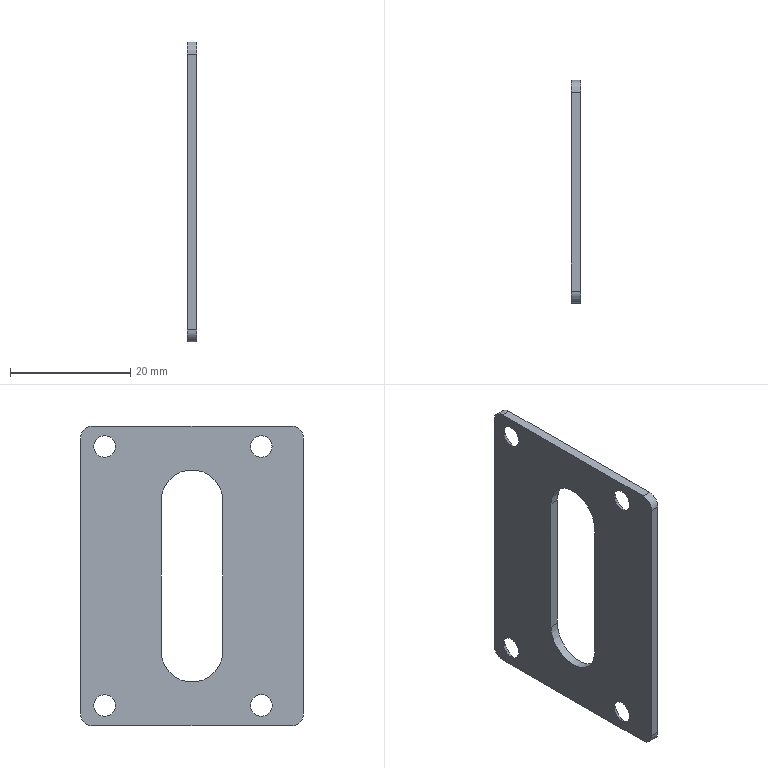Part | SolidWorks | features BaseBody 1, ICE 1 | 1 solid | 22 faces | box 1.5 x 37 x 49.8 mm | volume 2125 mm3 | cone 8 | plane 8 | cylinder 6 | commonest cylinder face diameters 4 x4 10.246 x2
STEP:
#1=CARTESIAN_POINT('',(0.,-2.2,3.4));
#2=VERTEX_POINT('',#1);
#3=CARTESIAN_POINT('',(0.,-5.8,3.4));
#4=VERTEX_POINT('',#3);
#5=CARTESIAN_POINT('',(0.,-4.,3.4));
#6=DIRECTION('',(-1.,0.,0.));
#7=DIRECTION('',(0.,1.,0.));
#8=AXIS2_PLACEMENT_3D('',#5,#6,#7);
#9=CIRCLE('',#8,1.8);
#10=EDGE_CURVE('',#2,#4,#9,.T.);
#11=ORIENTED_EDGE('',*,*,#10,.T.);
#12=CARTESIAN_POINT('',(1.5,-7.3,3.4));
#13=VERTEX_POINT('',#12);
#14=CARTESIAN_POINT('',(1.5,-7.3,3.4));
#15=DIRECTION('',(0.7071,-0.7071,0.));
#16=VECTOR('',#15,1000.);
#17=LINE('',#14,#16);
#18=EDGE_CURVE('',#4,#13,#17,.T.);
#19=ORIENTED_EDGE('',*,*,#18,.T.);
#20=CARTESIAN_POINT('',(1.5,-0.7,3.4));
#21=VERTEX_POINT('',#20);
#22=CARTESIAN_POINT('',(1.5,-4.,3.4));
#23=DIRECTION('',(-1.,0.,0.));
#24=DIRECTION('',(0.,1.,0.));
#25=AXIS2_PLACEMENT_3D('',#22,#23,#24);
#26=CIRCLE('',#25,3.3);
#27=EDGE_CURVE('',#21,#13,#26,.T.);
#28=ORIENTED_EDGE('',*,*,#27,.F.);
#29=CARTESIAN_POINT('',(1.5,-0.7,3.4));
#30=DIRECTION('',(0.7071,0.7071,0.));
#31=VECTOR('',#30,1000.);
#32=LINE('',#29,#31);
#33=EDGE_CURVE('',#2,#21,#32,.T.);
#34=ORIENTED_EDGE('',*,*,#33,.F.);
#35=EDGE_LOOP('',(#11,#19,#28,#34));
#36=FACE_OUTER_BOUND('',#35,.T.);
#37=CARTESIAN_POINT('',(1.5,-4.,3.4));
#38=DIRECTION('',(1.,0.,0.));
#39=DIRECTION('',(0.,1.,0.));
#40=AXIS2_PLACEMENT_3D('',#37,#38,#39);
#41=CONICAL_SURFACE('',#40,3.3,0.7854);
#42=ADVANCED_FACE('',(#36),#41,.F.);
#43=CARTESIAN_POINT('',(0.,-2.2,46.4));
#44=VERTEX_POINT('',#43);
#45=CARTESIAN_POINT('',(0.,-5.8,46.4));
#46=VERTEX_POINT('',#45);
#47=CARTESIAN_POINT('',(0.,-4.,46.4));
#48=DIRECTION('',(-1.,0.,0.));
#49=DIRECTION('',(0.,1.,0.));
#50=AXIS2_PLACEMENT_3D('',#47,#48,#49);
#51=CIRCLE('',#50,1.8);
#52=EDGE_CURVE('',#44,#46,#51,.T.);
#53=ORIENTED_EDGE('',*,*,#52,.T.);
#54=CARTESIAN_POINT('',(1.5,-7.3,46.4));
#55=VERTEX_POINT('',#54);
#56=CARTESIAN_POINT('',(1.5,-7.3,46.4));
#57=DIRECTION('',(0.7071,-0.7071,0.));
#58=VECTOR('',#57,1000.);
#59=LINE('',#56,#58);
#60=EDGE_CURVE('',#46,#55,#59,.T.);
#61=ORIENTED_EDGE('',*,*,#60,.T.);
#62=CARTESIAN_POINT('',(1.5,-0.7,46.4));
#63=VERTEX_POINT('',#62);
#64=CARTESIAN_POINT('',(1.5,-4.,46.4));
#65=DIRECTION('',(-1.,0.,0.));
#66=DIRECTION('',(0.,1.,0.));
#67=AXIS2_PLACEMENT_3D('',#64,#65,#66);
#68=CIRCLE('',#67,3.3);
#69=EDGE_CURVE('',#63,#55,#68,.T.);
#70=ORIENTED_EDGE('',*,*,#69,.F.);
#71=CARTESIAN_POINT('',(1.5,-0.7,46.4));
#72=DIRECTION('',(0.7071,0.7071,0.));
#73=VECTOR('',#72,1000.);
#74=LINE('',#71,#73);
#75=EDGE_CURVE('',#44,#63,#74,.T.);
#76=ORIENTED_EDGE('',*,*,#75,.F.);
#77=EDGE_LOOP('',(#53,#61,#70,#76));
#78=FACE_OUTER_BOUND('',#77,.T.);
#79=CARTESIAN_POINT('',(1.5,-4.,46.4));
#80=DIRECTION('',(1.,0.,0.));
#81=DIRECTION('',(0.,1.,0.));
#82=AXIS2_PLACEMENT_3D('',#79,#80,#81);
#83=CONICAL_SURFACE('',#82,3.3,0.7854);
#84=ADVANCED_FACE('',(#78),#83,.F.);
#85=CARTESIAN_POINT('',(0.,-28.2,46.4));
#86=VERTEX_POINT('',#85);
#87=CARTESIAN_POINT('',(0.,-31.8,46.4));
#88=VERTEX_POINT('',#87);
#89=CARTESIAN_POINT('',(0.,-30.,46.4));
#90=DIRECTION('',(-1.,0.,0.));
#91=DIRECTION('',(0.,1.,0.));
#92=AXIS2_PLACEMENT_3D('',#89,#90,#91);
#93=CIRCLE('',#92,1.8);
#94=EDGE_CURVE('',#86,#88,#93,.T.);
#95=ORIENTED_EDGE('',*,*,#94,.T.);
#96=CARTESIAN_POINT('',(1.5,-33.3,46.4));
#97=VERTEX_POINT('',#96);
#98=CARTESIAN_POINT('',(1.5,-33.3,46.4));
#99=DIRECTION('',(0.7071,-0.7071,0.));
#100=VECTOR('',#99,1000.);
#101=LINE('',#98,#100);
#102=EDGE_CURVE('',#88,#97,#101,.T.);
#103=ORIENTED_EDGE('',*,*,#102,.T.);
#104=CARTESIAN_POINT('',(1.5,-26.7,46.4));
#105=VERTEX_POINT('',#104);
#106=CARTESIAN_POINT('',(1.5,-30.,46.4));
#107=DIRECTION('',(-1.,0.,0.));
#108=DIRECTION('',(0.,1.,0.));
#109=AXIS2_PLACEMENT_3D('',#106,#107,#108);
#110=CIRCLE('',#109,3.3);
#111=EDGE_CURVE('',#105,#97,#110,.T.);
#112=ORIENTED_EDGE('',*,*,#111,.F.);
#113=CARTESIAN_POINT('',(1.5,-26.7,46.4));
#114=DIRECTION('',(0.7071,0.7071,0.));
#115=VECTOR('',#114,1000.);
#116=LINE('',#113,#115);
#117=EDGE_CURVE('',#86,#105,#116,.T.);
#118=ORIENTED_EDGE('',*,*,#117,.F.);
#119=EDGE_LOOP('',(#95,#103,#112,#118));
#120=FACE_OUTER_BOUND('',#119,.T.);
#121=CARTESIAN_POINT('',(1.5,-30.,46.4));
#122=DIRECTION('',(1.,0.,0.));
#123=DIRECTION('',(0.,1.,0.));
#124=AXIS2_PLACEMENT_3D('',#121,#122,#123);
#125=CONICAL_SURFACE('',#124,3.3,0.7854);
#126=ADVANCED_FACE('',(#120),#125,.F.);
#127=CARTESIAN_POINT('',(0.,-30.,1.6));
#128=VERTEX_POINT('',#127);
#129=CARTESIAN_POINT('',(0.,-30.,5.2));
#130=VERTEX_POINT('',#129);
#131=CARTESIAN_POINT('',(0.,-30.,3.4));
#132=DIRECTION('',(-1.,0.,0.));
#133=DIRECTION('',(0.,0.,-1.));
#134=AXIS2_PLACEMENT_3D('',#131,#132,#133);
#135=CIRCLE('',#134,1.8);
#136=EDGE_CURVE('',#128,#130,#135,.T.);
#137=ORIENTED_EDGE('',*,*,#136,.T.);
#138=CARTESIAN_POINT('',(1.5,-30.,6.7));
#139=VERTEX_POINT('',#138);
#140=CARTESIAN_POINT('',(1.5,-30.,6.7));
#141=DIRECTION('',(0.7071,0.,0.7071));
#142=VECTOR('',#141,1000.);
#143=LINE('',#140,#142);
#144=EDGE_CURVE('',#130,#139,#143,.T.);
#145=ORIENTED_EDGE('',*,*,#144,.T.);
#146=CARTESIAN_POINT('',(1.5,-30.,0.1));
#147=VERTEX_POINT('',#146);
#148=CARTESIAN_POINT('',(1.5,-30.,3.4));
#149=DIRECTION('',(-1.,0.,0.));
#150=DIRECTION('',(0.,0.,-1.));
#151=AXIS2_PLACEMENT_3D('',#148,#149,#150);
#152=CIRCLE('',#151,3.3);
#153=EDGE_CURVE('',#147,#139,#152,.T.);
#154=ORIENTED_EDGE('',*,*,#153,.F.);
#155=CARTESIAN_POINT('',(1.5,-30.,0.1));
#156=DIRECTION('',(0.7071,0.,-0.7071));
#157=VECTOR('',#156,1000.);
#158=LINE('',#155,#157);
#159=EDGE_CURVE('',#128,#147,#158,.T.);
#160=ORIENTED_EDGE('',*,*,#159,.F.);
#161=EDGE_LOOP('',(#137,#145,#154,#160));
#162=FACE_OUTER_BOUND('',#161,.T.);
#163=CARTESIAN_POINT('',(1.5,-30.,3.4));
#164=DIRECTION('',(1.,0.,0.));
#165=DIRECTION('',(0.,0.,-1.));
#166=AXIS2_PLACEMENT_3D('',#163,#164,#165);
#167=CONICAL_SURFACE('',#166,3.3,0.7854);
#168=ADVANCED_FACE('',(#162),#167,.F.);
#169=CARTESIAN_POINT('',(0.,-13.377,12.4));
#170=VERTEX_POINT('',#169);
#171=CARTESIAN_POINT('',(0.,-13.377,37.4));
#172=VERTEX_POINT('',#171);
#173=CARTESIAN_POINT('',(0.,-13.377,37.4));
#174=DIRECTION('',(0.,0.,1.));
#175=VECTOR('',#174,1000.);
#176=LINE('',#173,#175);
#177=EDGE_CURVE('',#170,#172,#176,.T.);
#178=ORIENTED_EDGE('',*,*,#177,.T.);
#179=CARTESIAN_POINT('',(0.,-23.623,37.4));
#180=VERTEX_POINT('',#179);
#181=CARTESIAN_POINT('',(0.,-18.5,37.4));
#182=DIRECTION('',(1.,0.,0.));
#183=DIRECTION('',(0.,1.,0.));
#184=AXIS2_PLACEMENT_3D('',#181,#182,#183);
#185=CIRCLE('',#184,5.123);
#186=EDGE_CURVE('',#172,#180,#185,.T.);
#187=ORIENTED_EDGE('',*,*,#186,.T.);
#188=CARTESIAN_POINT('',(0.,-23.623,12.4));
#189=VERTEX_POINT('',#188);
#190=CARTESIAN_POINT('',(0.,-23.623,37.4));
#191=DIRECTION('',(0.,0.,-1.));
#192=VECTOR('',#191,1000.);
#193=LINE('',#190,#192);
#194=EDGE_CURVE('',#180,#189,#193,.T.);
#195=ORIENTED_EDGE('',*,*,#194,.T.);
#196=CARTESIAN_POINT('',(0.,-18.5,12.4));
#197=DIRECTION('',(1.,0.,0.));
#198=DIRECTION('',(0.,1.,0.));
#199=AXIS2_PLACEMENT_3D('',#196,#197,#198);
#200=CIRCLE('',#199,5.123);
#201=EDGE_CURVE('',#189,#170,#200,.T.);
#202=ORIENTED_EDGE('',*,*,#201,.T.);
#203=EDGE_LOOP('',(#178,#187,#195,#202));
#204=FACE_BOUND('',#203,.T.);
#205=CARTESIAN_POINT('',(0.,-37.,2.));
#206=VERTEX_POINT('',#205);
#207=CARTESIAN_POINT('',(0.,-35.,0.));
#208=VERTEX_POINT('',#207);
#209=CARTESIAN_POINT('',(0.,-35.,2.));
#210=DIRECTION('',(1.,0.,0.));
#211=DIRECTION('',(0.,0.,1.));
#212=AXIS2_PLACEMENT_3D('',#209,#210,#211);
#213=CIRCLE('',#212,2.);
#214=EDGE_CURVE('',#206,#208,#213,.T.);
#215=ORIENTED_EDGE('',*,*,#214,.F.);
#216=CARTESIAN_POINT('',(0.,-37.,47.8));
#217=VERTEX_POINT('',#216);
#218=CARTESIAN_POINT('',(0.,-37.,49.8));
#219=DIRECTION('',(0.,0.,-1.));
#220=VECTOR('',#219,1000.);
#221=LINE('',#218,#220);
#222=EDGE_CURVE('',#217,#206,#221,.T.);
#223=ORIENTED_EDGE('',*,*,#222,.F.);
#224=CARTESIAN_POINT('',(0.,-35.,49.8));
#225=VERTEX_POINT('',#224);
#226=CARTESIAN_POINT('',(0.,-35.,47.8));
#227=DIRECTION('',(1.,0.,0.));
#228=DIRECTION('',(0.,0.,-1.));
#229=AXIS2_PLACEMENT_3D('',#226,#227,#228);
#230=CIRCLE('',#229,2.);
#231=EDGE_CURVE('',#225,#217,#230,.T.);
#232=ORIENTED_EDGE('',*,*,#231,.F.);
#233=CARTESIAN_POINT('',(0.,-2.,49.8));
#234=VERTEX_POINT('',#233);
#235=CARTESIAN_POINT('',(0.,-37.,49.8));
#236=DIRECTION('',(0.,-1.,0.));
#237=VECTOR('',#236,1000.);
#238=LINE('',#235,#237);
#239=EDGE_CURVE('',#234,#225,#238,.T.);
#240=ORIENTED_EDGE('',*,*,#239,.F.);
#241=CARTESIAN_POINT('',(0.,0.,47.8));
#242=VERTEX_POINT('',#241);
#243=CARTESIAN_POINT('',(0.,-2.,47.8));
#244=DIRECTION('',(1.,0.,0.));
#245=DIRECTION('',(0.,-1.,0.));
#246=AXIS2_PLACEMENT_3D('',#243,#244,#245);
#247=CIRCLE('',#246,2.);
#248=EDGE_CURVE('',#242,#234,#247,.T.);
#249=ORIENTED_EDGE('',*,*,#248,.F.);
#250=CARTESIAN_POINT('',(0.,0.,2.));
#251=VERTEX_POINT('',#250);
#252=CARTESIAN_POINT('',(0.,0.,49.8));
#253=DIRECTION('',(0.,0.,1.));
#254=VECTOR('',#253,1000.);
#255=LINE('',#252,#254);
#256=EDGE_CURVE('',#251,#242,#255,.T.);
#257=ORIENTED_EDGE('',*,*,#256,.F.);
#258=CARTESIAN_POINT('',(0.,-2.,0.));
#259=VERTEX_POINT('',#258);
#260=CARTESIAN_POINT('',(0.,-2.,2.));
#261=DIRECTION('',(1.,0.,0.));
#262=DIRECTION('',(0.,1.,0.));
#263=AXIS2_PLACEMENT_3D('',#260,#261,#262);
#264=CIRCLE('',#263,2.);
#265=EDGE_CURVE('',#259,#251,#264,.T.);
#266=ORIENTED_EDGE('',*,*,#265,.F.);
#267=CARTESIAN_POINT('',(0.,-37.,0.));
#268=DIRECTION('',(0.,1.,0.));
#269=VECTOR('',#268,1000.);
#270=LINE('',#267,#269);
#271=EDGE_CURVE('',#208,#259,#270,.T.);
#272=ORIENTED_EDGE('',*,*,#271,.F.);
#273=EDGE_LOOP('',(#215,#223,#232,#240,#249,#257,#266,#272));
#274=FACE_OUTER_BOUND('',#273,.T.);
#275=ORIENTED_EDGE('',*,*,#10,.F.);
#276=CARTESIAN_POINT('',(0.,-4.,3.4));
#277=DIRECTION('',(-1.,0.,0.));
#278=DIRECTION('',(0.,1.,0.));
#279=AXIS2_PLACEMENT_3D('',#276,#277,#278);
#280=CIRCLE('',#279,1.8);
#281=EDGE_CURVE('',#4,#2,#280,.T.);
#282=ORIENTED_EDGE('',*,*,#281,.F.);
#283=EDGE_LOOP('',(#275,#282));
#284=FACE_BOUND('',#283,.T.);
#285=ORIENTED_EDGE('',*,*,#52,.F.);
#286=CARTESIAN_POINT('',(0.,-4.,46.4));
#287=DIRECTION('',(-1.,0.,0.));
#288=DIRECTION('',(0.,1.,0.));
#289=AXIS2_PLACEMENT_3D('',#286,#287,#288);
#290=CIRCLE('',#289,1.8);
#291=EDGE_CURVE('',#46,#44,#290,.T.);
#292=ORIENTED_EDGE('',*,*,#291,.F.);
#293=EDGE_LOOP('',(#285,#292));
#294=FACE_BOUND('',#293,.T.);
#295=ORIENTED_EDGE('',*,*,#94,.F.);
#296=CARTESIAN_POINT('',(0.,-30.,46.4));
#297=DIRECTION('',(-1.,0.,0.));
#298=DIRECTION('',(0.,1.,0.));
#299=AXIS2_PLACEMENT_3D('',#296,#297,#298);
#300=CIRCLE('',#299,1.8);
#301=EDGE_CURVE('',#88,#86,#300,.T.);
#302=ORIENTED_EDGE('',*,*,#301,.F.);
#303=EDGE_LOOP('',(#295,#302));
#304=FACE_BOUND('',#303,.T.);
#305=ORIENTED_EDGE('',*,*,#136,.F.);
#306=CARTESIAN_POINT('',(0.,-30.,3.4));
#307=DIRECTION('',(-1.,0.,0.));
#308=DIRECTION('',(0.,0.,-1.));
#309=AXIS2_PLACEMENT_3D('',#306,#307,#308);
#310=CIRCLE('',#309,1.8);
#311=EDGE_CURVE('',#130,#128,#310,.T.);
#312=ORIENTED_EDGE('',*,*,#311,.F.);
#313=EDGE_LOOP('',(#305,#312));
#314=FACE_BOUND('',#313,.T.);
#315=CARTESIAN_POINT('',(0.,-37.,49.8));
#316=DIRECTION('',(1.,0.,0.));
#317=DIRECTION('',(0.,1.,0.));
#318=AXIS2_PLACEMENT_3D('',#315,#316,#317);
#319=PLANE('',#318);
#320=ADVANCED_FACE('',(#204,#274,#284,#294,#304,#314),#319,.F.);
#321=ORIENTED_EDGE('',*,*,#271,.T.);
#322=CARTESIAN_POINT('',(1.5,-2.,0.));
#323=VERTEX_POINT('',#322);
#324=CARTESIAN_POINT('',(0.,-2.,0.));
#325=DIRECTION('',(1.,0.,0.));
#326=VECTOR('',#325,1000.);
#327=LINE('',#324,#326);
#328=EDGE_CURVE('',#259,#323,#327,.T.);
#329=ORIENTED_EDGE('',*,*,#328,.T.);
#330=CARTESIAN_POINT('',(1.5,-35.,0.));
#331=VERTEX_POINT('',#330);
#332=CARTESIAN_POINT('',(1.5,0.,0.));
#333=DIRECTION('',(0.,-1.,0.));
#334=VECTOR('',#333,1000.);
#335=LINE('',#332,#334);
#336=EDGE_CURVE('',#323,#331,#335,.T.);
#337=ORIENTED_EDGE('',*,*,#336,.T.);
#338=CARTESIAN_POINT('',(0.,-35.,0.));
#339=DIRECTION('',(-1.,0.,0.));
#340=VECTOR('',#339,1000.);
#341=LINE('',#338,#340);
#342=EDGE_CURVE('',#331,#208,#341,.T.);
#343=ORIENTED_EDGE('',*,*,#342,.T.);
#344=EDGE_LOOP('',(#321,#329,#337,#343));
#345=FACE_OUTER_BOUND('',#344,.T.);
#346=CARTESIAN_POINT('',(0.,0.,0.));
#347=DIRECTION('',(0.,0.,-1.));
#348=DIRECTION('',(-1.,0.,0.));
#349=AXIS2_PLACEMENT_3D('',#346,#347,#348);
#350=PLANE('',#349);
#351=ADVANCED_FACE('',(#345),#350,.T.);
#352=CARTESIAN_POINT('',(1.5,-37.,2.));
#353=VERTEX_POINT('',#352);
#354=CARTESIAN_POINT('',(1.5,-35.,2.));
#355=DIRECTION('',(-1.,0.,0.));
#356=DIRECTION('',(0.,0.,1.));
#357=AXIS2_PLACEMENT_3D('',#354,#355,#356);
#358=CIRCLE('',#357,2.);
#359=EDGE_CURVE('',#331,#353,#358,.T.);
#360=ORIENTED_EDGE('',*,*,#359,.T.);
#361=CARTESIAN_POINT('',(1.5,-37.,2.));
#362=DIRECTION('',(-1.,0.,0.));
#363=VECTOR('',#362,1000.);
#364=LINE('',#361,#363);
#365=EDGE_CURVE('',#353,#206,#364,.T.);
#366=ORIENTED_EDGE('',*,*,#365,.T.);
#367=ORIENTED_EDGE('',*,*,#214,.T.);
#368=ORIENTED_EDGE('',*,*,#342,.F.);
#369=EDGE_LOOP('',(#360,#366,#367,#368));
#370=FACE_OUTER_BOUND('',#369,.T.);
#371=CARTESIAN_POINT('',(1.5,-35.,2.));
#372=DIRECTION('',(-1.,0.,0.));
#373=DIRECTION('',(0.,0.,1.));
#374=AXIS2_PLACEMENT_3D('',#371,#372,#373);
#375=CYLINDRICAL_SURFACE('',#374,2.);
#376=ADVANCED_FACE('',(#370),#375,.T.);
#377=ORIENTED_EDGE('',*,*,#365,.F.);
#378=CARTESIAN_POINT('',(1.5,-37.,47.8));
#379=VERTEX_POINT('',#378);
#380=CARTESIAN_POINT('',(1.5,-37.,49.8));
#381=DIRECTION('',(0.,0.,-1.));
#382=VECTOR('',#381,1000.);
#383=LINE('',#380,#382);
#384=EDGE_CURVE('',#379,#353,#383,.T.);
#385=ORIENTED_EDGE('',*,*,#384,.F.);
#386=CARTESIAN_POINT('',(1.5,-37.,47.8));
#387=DIRECTION('',(1.,0.,0.));
#388=VECTOR('',#387,1000.);
#389=LINE('',#386,#388);
#390=EDGE_CURVE('',#217,#379,#389,.T.);
#391=ORIENTED_EDGE('',*,*,#390,.F.);
#392=ORIENTED_EDGE('',*,*,#222,.T.);
#393=EDGE_LOOP('',(#377,#385,#391,#392));
#394=FACE_OUTER_BOUND('',#393,.T.);
#395=CARTESIAN_POINT('',(1.5,-37.,49.8));
#396=DIRECTION('',(0.,1.,0.));
#397=DIRECTION('',(0.,0.,1.));
#398=AXIS2_PLACEMENT_3D('',#395,#396,#397);
#399=PLANE('',#398);
#400=ADVANCED_FACE('',(#394),#399,.F.);
#401=CARTESIAN_POINT('',(1.5,-35.,49.8));
#402=VERTEX_POINT('',#401);
#403=CARTESIAN_POINT('',(1.5,-35.,47.8));
#404=DIRECTION('',(-1.,0.,0.));
#405=DIRECTION('',(0.,0.,-1.));
#406=AXIS2_PLACEMENT_3D('',#403,#404,#405);
#407=CIRCLE('',#406,2.);
#408=EDGE_CURVE('',#379,#402,#407,.T.);
#409=ORIENTED_EDGE('',*,*,#408,.T.);
#410=CARTESIAN_POINT('',(0.,-35.,49.8));
#411=DIRECTION('',(-1.,0.,0.));
#412=VECTOR('',#411,1000.);
#413=LINE('',#410,#412);
#414=EDGE_CURVE('',#402,#225,#413,.T.);
#415=ORIENTED_EDGE('',*,*,#414,.T.);
#416=ORIENTED_EDGE('',*,*,#231,.T.);
#417=ORIENTED_EDGE('',*,*,#390,.T.);
#418=EDGE_LOOP('',(#409,#415,#416,#417));
#419=FACE_OUTER_BOUND('',#418,.T.);
#420=CARTESIAN_POINT('',(0.,-35.,47.8));
#421=DIRECTION('',(1.,0.,0.));
#422=DIRECTION('',(0.,0.,-1.));
#423=AXIS2_PLACEMENT_3D('',#420,#421,#422);
#424=CYLINDRICAL_SURFACE('',#423,2.);
#425=ADVANCED_FACE('',(#419),#424,.T.);
#426=ORIENTED_EDGE('',*,*,#414,.F.);
#427=CARTESIAN_POINT('',(1.5,-2.,49.8));
#428=VERTEX_POINT('',#427);
#429=CARTESIAN_POINT('',(1.5,0.,49.8));
#430=DIRECTION('',(0.,-1.,0.));
#431=VECTOR('',#430,1000.);
#432=LINE('',#429,#431);
#433=EDGE_CURVE('',#428,#402,#432,.T.);
#434=ORIENTED_EDGE('',*,*,#433,.F.);
#435=CARTESIAN_POINT('',(0.,-2.,49.8));
#436=DIRECTION('',(1.,0.,0.));
#437=VECTOR('',#436,1000.);
#438=LINE('',#435,#437);
#439=EDGE_CURVE('',#234,#428,#438,.T.);
#440=ORIENTED_EDGE('',*,*,#439,.F.);
#441=ORIENTED_EDGE('',*,*,#239,.T.);
#442=EDGE_LOOP('',(#426,#434,#440,#441));
#443=FACE_OUTER_BOUND('',#442,.T.);
#444=CARTESIAN_POINT('',(0.,0.,49.8));
#445=DIRECTION('',(0.,0.,-1.));
#446=DIRECTION('',(-1.,0.,0.));
#447=AXIS2_PLACEMENT_3D('',#444,#445,#446);
#448=PLANE('',#447);
#449=ADVANCED_FACE('',(#443),#448,.F.);
#450=ORIENTED_EDGE('',*,*,#248,.T.);
#451=ORIENTED_EDGE('',*,*,#439,.T.);
#452=CARTESIAN_POINT('',(1.5,0.,47.8));
#453=VERTEX_POINT('',#452);
#454=CARTESIAN_POINT('',(1.5,-2.,47.8));
#455=DIRECTION('',(-1.,0.,0.));
#456=DIRECTION('',(0.,-1.,0.));
#457=AXIS2_PLACEMENT_3D('',#454,#455,#456);
#458=CIRCLE('',#457,2.);
#459=EDGE_CURVE('',#428,#453,#458,.T.);
#460=ORIENTED_EDGE('',*,*,#459,.T.);
#461=CARTESIAN_POINT('',(0.,0.,47.8));
#462=DIRECTION('',(-1.,0.,0.));
#463=VECTOR('',#462,1000.);
#464=LINE('',#461,#463);
#465=EDGE_CURVE('',#453,#242,#464,.T.);
#466=ORIENTED_EDGE('',*,*,#465,.T.);
#467=EDGE_LOOP('',(#450,#451,#460,#466));
#468=FACE_OUTER_BOUND('',#467,.T.);
#469=CARTESIAN_POINT('',(0.,-2.,47.8));
#470=DIRECTION('',(-1.,0.,0.));
#471=DIRECTION('',(0.,-1.,0.));
#472=AXIS2_PLACEMENT_3D('',#469,#470,#471);
#473=CYLINDRICAL_SURFACE('',#472,2.);
#474=ADVANCED_FACE('',(#468),#473,.T.);
#475=ORIENTED_EDGE('',*,*,#465,.F.);
#476=CARTESIAN_POINT('',(1.5,0.,2.));
#477=VERTEX_POINT('',#476);
#478=CARTESIAN_POINT('',(1.5,0.,49.8));
#479=DIRECTION('',(0.,0.,1.));
#480=VECTOR('',#479,1000.);
#481=LINE('',#478,#480);
#482=EDGE_CURVE('',#477,#453,#481,.T.);
#483=ORIENTED_EDGE('',*,*,#482,.F.);
#484=CARTESIAN_POINT('',(0.,0.,2.));
#485=DIRECTION('',(1.,0.,0.));
#486=VECTOR('',#485,1000.);
#487=LINE('',#484,#486);
#488=EDGE_CURVE('',#251,#477,#487,.T.);
#489=ORIENTED_EDGE('',*,*,#488,.F.);
#490=ORIENTED_EDGE('',*,*,#256,.T.);
#491=EDGE_LOOP('',(#475,#483,#489,#490));
#492=FACE_OUTER_BOUND('',#491,.T.);
#493=CARTESIAN_POINT('',(0.,0.,49.8));
#494=DIRECTION('',(0.,-1.,0.));
#495=DIRECTION('',(1.,0.,0.));
#496=AXIS2_PLACEMENT_3D('',#493,#494,#495);
#497=PLANE('',#496);
#498=ADVANCED_FACE('',(#492),#497,.F.);
#499=ORIENTED_EDGE('',*,*,#265,.T.);
#500=ORIENTED_EDGE('',*,*,#488,.T.);
#501=CARTESIAN_POINT('',(1.5,-2.,2.));
#502=DIRECTION('',(-1.,0.,0.));
#503=DIRECTION('',(0.,1.,0.));
#504=AXIS2_PLACEMENT_3D('',#501,#502,#503);
#505=CIRCLE('',#504,2.);
#506=EDGE_CURVE('',#477,#323,#505,.T.);
#507=ORIENTED_EDGE('',*,*,#506,.T.);
#508=ORIENTED_EDGE('',*,*,#328,.F.);
#509=EDGE_LOOP('',(#499,#500,#507,#508));
#510=FACE_OUTER_BOUND('',#509,.T.);
#511=CARTESIAN_POINT('',(0.,-2.,2.));
#512=DIRECTION('',(1.,0.,0.));
#513=DIRECTION('',(0.,1.,0.));
#514=AXIS2_PLACEMENT_3D('',#511,#512,#513);
#515=CYLINDRICAL_SURFACE('',#514,2.);
#516=ADVANCED_FACE('',(#510),#515,.T.);
#517=ORIENTED_EDGE('',*,*,#18,.F.);
#518=ORIENTED_EDGE('',*,*,#281,.T.);
#519=ORIENTED_EDGE('',*,*,#33,.T.);
#520=CARTESIAN_POINT('',(1.5,-4.,3.4));
#521=DIRECTION('',(-1.,0.,0.));
#522=DIRECTION('',(0.,1.,0.));
#523=AXIS2_PLACEMENT_3D('',#520,#521,#522);
#524=CIRCLE('',#523,3.3);
#525=EDGE_CURVE('',#13,#21,#524,.T.);
#526=ORIENTED_EDGE('',*,*,#525,.F.);
#527=EDGE_LOOP('',(#517,#518,#519,#526));
#528=FACE_OUTER_BOUND('',#527,.T.);
#529=CARTESIAN_POINT('',(1.5,-4.,3.4));
#530=DIRECTION('',(1.,0.,0.));
#531=DIRECTION('',(0.,1.,0.));
#532=AXIS2_PLACEMENT_3D('',#529,#530,#531);
#533=CONICAL_SURFACE('',#532,3.3,0.7854);
#534=ADVANCED_FACE('',(#528),#533,.F.);
#535=ORIENTED_EDGE('',*,*,#60,.F.);
#536=ORIENTED_EDGE('',*,*,#291,.T.);
#537=ORIENTED_EDGE('',*,*,#75,.T.);
#538=CARTESIAN_POINT('',(1.5,-4.,46.4));
#539=DIRECTION('',(-1.,0.,0.));
#540=DIRECTION('',(0.,1.,0.));
#541=AXIS2_PLACEMENT_3D('',#538,#539,#540);
#542=CIRCLE('',#541,3.3);
#543=EDGE_CURVE('',#55,#63,#542,.T.);
#544=ORIENTED_EDGE('',*,*,#543,.F.);
#545=EDGE_LOOP('',(#535,#536,#537,#544));
#546=FACE_OUTER_BOUND('',#545,.T.);
#547=CARTESIAN_POINT('',(1.5,-4.,46.4));
#548=DIRECTION('',(1.,0.,0.));
#549=DIRECTION('',(0.,1.,0.));
#550=AXIS2_PLACEMENT_3D('',#547,#548,#549);
#551=CONICAL_SURFACE('',#550,3.3,0.7854);
#552=ADVANCED_FACE('',(#546),#551,.F.);
#553=ORIENTED_EDGE('',*,*,#102,.F.);
#554=ORIENTED_EDGE('',*,*,#301,.T.);
#555=ORIENTED_EDGE('',*,*,#117,.T.);
#556=CARTESIAN_POINT('',(1.5,-30.,46.4));
#557=DIRECTION('',(-1.,0.,0.));
#558=DIRECTION('',(0.,1.,0.));
#559=AXIS2_PLACEMENT_3D('',#556,#557,#558);
#560=CIRCLE('',#559,3.3);
#561=EDGE_CURVE('',#97,#105,#560,.T.);
#562=ORIENTED_EDGE('',*,*,#561,.F.);
#563=EDGE_LOOP('',(#553,#554,#555,#562));
#564=FACE_OUTER_BOUND('',#563,.T.);
#565=CARTESIAN_POINT('',(1.5,-30.,46.4));
#566=DIRECTION('',(1.,0.,0.));
#567=DIRECTION('',(0.,1.,0.));
#568=AXIS2_PLACEMENT_3D('',#565,#566,#567);
#569=CONICAL_SURFACE('',#568,3.3,0.7854);
#570=ADVANCED_FACE('',(#564),#569,.F.);
#571=ORIENTED_EDGE('',*,*,#144,.F.);
#572=ORIENTED_EDGE('',*,*,#311,.T.);
#573=ORIENTED_EDGE('',*,*,#159,.T.);
#574=CARTESIAN_POINT('',(1.5,-30.,3.4));
#575=DIRECTION('',(-1.,0.,0.));
#576=DIRECTION('',(0.,0.,-1.));
#577=AXIS2_PLACEMENT_3D('',#574,#575,#576);
#578=CIRCLE('',#577,3.3);
#579=EDGE_CURVE('',#139,#147,#578,.T.);
#580=ORIENTED_EDGE('',*,*,#579,.F.);
#581=EDGE_LOOP('',(#571,#572,#573,#580));
#582=FACE_OUTER_BOUND('',#581,.T.);
#583=CARTESIAN_POINT('',(1.5,-30.,3.4));
#584=DIRECTION('',(1.,0.,0.));
#585=DIRECTION('',(0.,0.,-1.));
#586=AXIS2_PLACEMENT_3D('',#583,#584,#585);
#587=CONICAL_SURFACE('',#586,3.3,0.7854);
#588=ADVANCED_FACE('',(#582),#587,.F.);
#589=CARTESIAN_POINT('',(1.5,-23.623,37.4));
#590=VERTEX_POINT('',#589);
#591=CARTESIAN_POINT('',(1.5,-23.623,12.4));
#592=VERTEX_POINT('',#591);
#593=CARTESIAN_POINT('',(1.5,-23.623,37.4));
#594=DIRECTION('',(0.,0.,-1.));
#595=VECTOR('',#594,1000.);
#596=LINE('',#593,#595);
#597=EDGE_CURVE('',#590,#592,#596,.T.);
#598=ORIENTED_EDGE('',*,*,#597,.F.);
#599=CARTESIAN_POINT('',(1.5,-13.377,37.4));
#600=VERTEX_POINT('',#599);
#601=CARTESIAN_POINT('',(1.5,-18.5,37.4));
#602=DIRECTION('',(1.,0.,0.));
#603=DIRECTION('',(0.,1.,0.));
#604=AXIS2_PLACEMENT_3D('',#601,#602,#603);
#605=CIRCLE('',#604,5.123);
#606=EDGE_CURVE('',#600,#590,#605,.T.);
#607=ORIENTED_EDGE('',*,*,#606,.F.);
#608=CARTESIAN_POINT('',(1.5,-13.377,12.4));
#609=VERTEX_POINT('',#608);
#610=CARTESIAN_POINT('',(1.5,-13.377,37.4));
#611=DIRECTION('',(0.,0.,1.));
#612=VECTOR('',#611,1000.);
#613=LINE('',#610,#612);
#614=EDGE_CURVE('',#609,#600,#613,.T.);
#615=ORIENTED_EDGE('',*,*,#614,.F.);
#616=CARTESIAN_POINT('',(1.5,-18.5,12.4));
#617=DIRECTION('',(1.,0.,0.));
#618=DIRECTION('',(0.,1.,0.));
#619=AXIS2_PLACEMENT_3D('',#616,#617,#618);
#620=CIRCLE('',#619,5.123);
#621=EDGE_CURVE('',#592,#609,#620,.T.);
#622=ORIENTED_EDGE('',*,*,#621,.F.);
#623=EDGE_LOOP('',(#598,#607,#615,#622));
#624=FACE_BOUND('',#623,.T.);
#625=ORIENTED_EDGE('',*,*,#359,.F.);
#626=ORIENTED_EDGE('',*,*,#336,.F.);
#627=ORIENTED_EDGE('',*,*,#506,.F.);
#628=ORIENTED_EDGE('',*,*,#482,.T.);
#629=ORIENTED_EDGE('',*,*,#459,.F.);
#630=ORIENTED_EDGE('',*,*,#433,.T.);
#631=ORIENTED_EDGE('',*,*,#408,.F.);
#632=ORIENTED_EDGE('',*,*,#384,.T.);
#633=EDGE_LOOP('',(#625,#626,#627,#628,#629,#630,#631,#632));
#634=FACE_OUTER_BOUND('',#633,.T.);
#635=ORIENTED_EDGE('',*,*,#27,.T.);
#636=ORIENTED_EDGE('',*,*,#525,.T.);
#637=EDGE_LOOP('',(#635,#636));
#638=FACE_BOUND('',#637,.T.);
#639=ORIENTED_EDGE('',*,*,#69,.T.);
#640=ORIENTED_EDGE('',*,*,#543,.T.);
#641=EDGE_LOOP('',(#639,#640));
#642=FACE_BOUND('',#641,.T.);
#643=ORIENTED_EDGE('',*,*,#111,.T.);
#644=ORIENTED_EDGE('',*,*,#561,.T.);
#645=EDGE_LOOP('',(#643,#644));
#646=FACE_BOUND('',#645,.T.);
#647=ORIENTED_EDGE('',*,*,#153,.T.);
#648=ORIENTED_EDGE('',*,*,#579,.T.);
#649=EDGE_LOOP('',(#647,#648));
#650=FACE_BOUND('',#649,.T.);
#651=CARTESIAN_POINT('',(1.5,0.,49.8));
#652=DIRECTION('',(-1.,0.,0.));
#653=DIRECTION('',(0.,-1.,0.));
#654=AXIS2_PLACEMENT_3D('',#651,#652,#653);
#655=PLANE('',#654);
#656=ADVANCED_FACE('',(#624,#634,#638,#642,#646,#650),#655,.F.);
#657=ORIENTED_EDGE('',*,*,#606,.T.);
#658=CARTESIAN_POINT('',(0.,-23.623,37.4));
#659=DIRECTION('',(1.,0.,0.));
#660=VECTOR('',#659,1000.);
#661=LINE('',#658,#660);
#662=EDGE_CURVE('',#180,#590,#661,.T.);
#663=ORIENTED_EDGE('',*,*,#662,.F.);
#664=ORIENTED_EDGE('',*,*,#186,.F.);
#665=CARTESIAN_POINT('',(0.,-13.377,37.4));
#666=DIRECTION('',(1.,0.,0.));
#667=VECTOR('',#666,1000.);
#668=LINE('',#665,#667);
#669=EDGE_CURVE('',#172,#600,#668,.T.);
#670=ORIENTED_EDGE('',*,*,#669,.T.);
#671=EDGE_LOOP('',(#657,#663,#664,#670));
#672=FACE_OUTER_BOUND('',#671,.T.);
#673=CARTESIAN_POINT('',(0.,-18.5,37.4));
#674=DIRECTION('',(1.,0.,0.));
#675=DIRECTION('',(0.,1.,0.));
#676=AXIS2_PLACEMENT_3D('',#673,#674,#675);
#677=CYLINDRICAL_SURFACE('',#676,5.123);
#678=ADVANCED_FACE('',(#672),#677,.F.);
#679=ORIENTED_EDGE('',*,*,#614,.T.);
#680=ORIENTED_EDGE('',*,*,#669,.F.);
#681=ORIENTED_EDGE('',*,*,#177,.F.);
#682=CARTESIAN_POINT('',(0.,-13.377,12.4));
#683=DIRECTION('',(1.,0.,0.));
#684=VECTOR('',#683,1000.);
#685=LINE('',#682,#684);
#686=EDGE_CURVE('',#170,#609,#685,.T.);
#687=ORIENTED_EDGE('',*,*,#686,.T.);
#688=EDGE_LOOP('',(#679,#680,#681,#687));
#689=FACE_OUTER_BOUND('',#688,.T.);
#690=CARTESIAN_POINT('',(0.,-13.377,37.4));
#691=DIRECTION('',(0.,1.,0.));
#692=DIRECTION('',(-1.,0.,0.));
#693=AXIS2_PLACEMENT_3D('',#690,#691,#692);
#694=PLANE('',#693);
#695=ADVANCED_FACE('',(#689),#694,.F.);
#696=ORIENTED_EDGE('',*,*,#621,.T.);
#697=ORIENTED_EDGE('',*,*,#686,.F.);
#698=ORIENTED_EDGE('',*,*,#201,.F.);
#699=CARTESIAN_POINT('',(0.,-23.623,12.4));
#700=DIRECTION('',(1.,0.,0.));
#701=VECTOR('',#700,1000.);
#702=LINE('',#699,#701);
#703=EDGE_CURVE('',#189,#592,#702,.T.);
#704=ORIENTED_EDGE('',*,*,#703,.T.);
#705=EDGE_LOOP('',(#696,#697,#698,#704));
#706=FACE_OUTER_BOUND('',#705,.T.);
#707=CARTESIAN_POINT('',(0.,-18.5,12.4));
#708=DIRECTION('',(1.,0.,0.));
#709=DIRECTION('',(0.,1.,0.));
#710=AXIS2_PLACEMENT_3D('',#707,#708,#709);
#711=CYLINDRICAL_SURFACE('',#710,5.123);
#712=ADVANCED_FACE('',(#706),#711,.F.);
#713=ORIENTED_EDGE('',*,*,#597,.T.);
#714=ORIENTED_EDGE('',*,*,#703,.F.);
#715=ORIENTED_EDGE('',*,*,#194,.F.);
#716=ORIENTED_EDGE('',*,*,#662,.T.);
#717=EDGE_LOOP('',(#713,#714,#715,#716));
#718=FACE_OUTER_BOUND('',#717,.T.);
#719=CARTESIAN_POINT('',(0.,-23.623,37.4));
#720=DIRECTION('',(0.,-1.,0.));
#721=DIRECTION('',(1.,0.,0.));
#722=AXIS2_PLACEMENT_3D('',#719,#720,#721);
#723=PLANE('',#722);
#724=ADVANCED_FACE('',(#718),#723,.F.);
#725=CLOSED_SHELL('',(#42,#84,#126,#168,#320,#351,#376,#400,#425,#449,#474,#498,#516,#534,#552,#570,#588,#656,#678,#695,#712,#724));
#726=MANIFOLD_SOLID_BREP('',#725);
#727=CARTESIAN_POINT('',(0.,0.,0.));
#728=DIRECTION('',(0.,0.,1.));
#729=DIRECTION('',(1.,0.,0.));
#730=AXIS2_PLACEMENT_3D('',#727,#728,#729);
#731=(LENGTH_UNIT()NAMED_UNIT(*)SI_UNIT(.MILLI.,.METRE.));
#732=UNCERTAINTY_MEASURE_WITH_UNIT(LENGTH_MEASURE(0.00001),#731,'','');
#733=(NAMED_UNIT(*)PLANE_ANGLE_UNIT()SI_UNIT($,.RADIAN.));
#734=(NAMED_UNIT(*)SI_UNIT($,.STERADIAN.)SOLID_ANGLE_UNIT());
#735=(GEOMETRIC_REPRESENTATION_CONTEXT(3)GLOBAL_UNCERTAINTY_ASSIGNED_CONTEXT((#732))GLOBAL_UNIT_ASSIGNED_CONTEXT((#731,#733,#734))REPRESENTATION_CONTEXT('',''));
#736=ADVANCED_BREP_SHAPE_REPRESENTATION('',(#726,#730),#735);